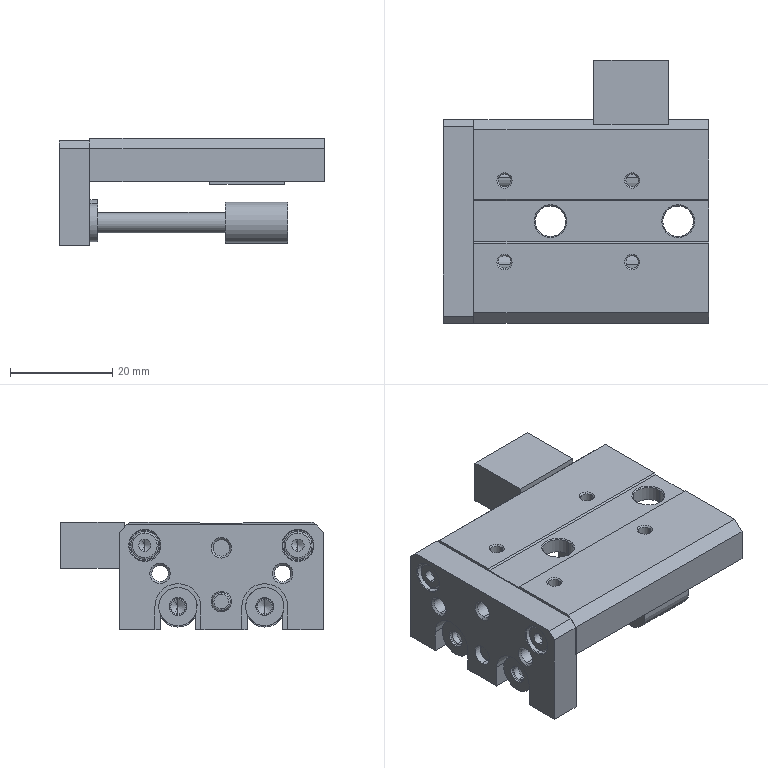Part | STEP file | HLQ8-10-S-AS-2-1 | 1 solid | 236 faces | box 52 x 51.5 x 21 mm | volume 19231 mm3 | cylinder 88 | plane 86 | cone 52 | spline 10 | commonest cylinder face diameters 2.459 x12 5.5 x12 6 x12 7.5 x8 3.242 x6 3.5 x6